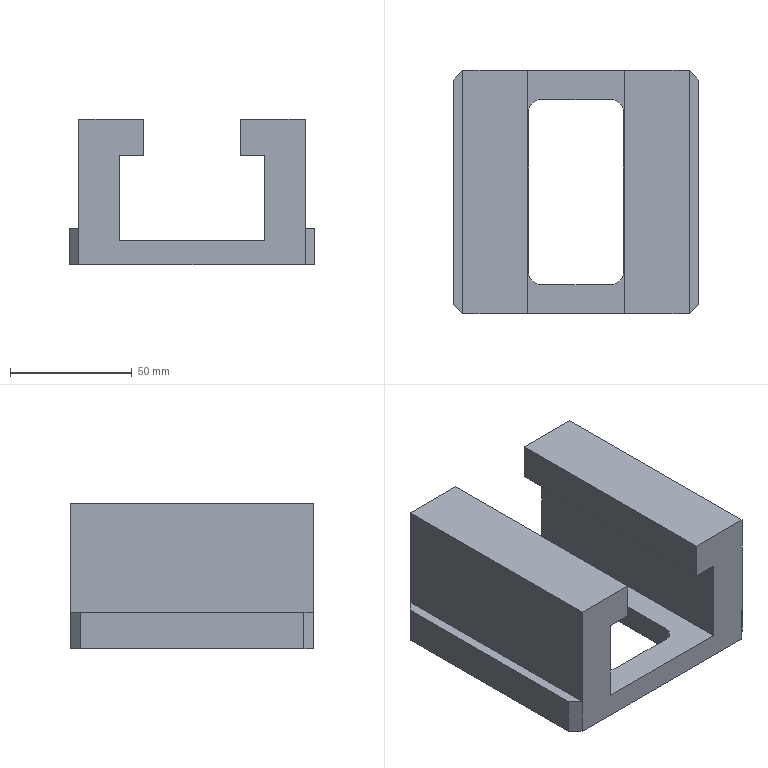Part | STEP file | solid 87 | 1 solid | 46 faces | box 101 x 100 x 60 mm | volume 261945 mm3 | plane 26 | cylinder 10 | cone 10 | commonest cylinder face diameters 10 x6 8.5 x4